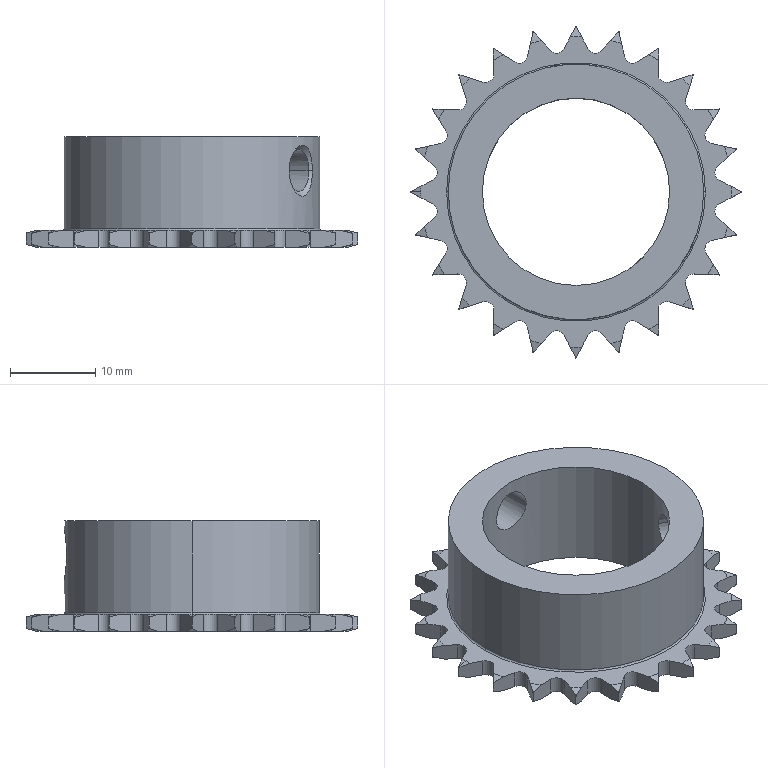Part | SolidWorks | features ICE 3, RevCut 2, Revolution 1 | 1 solid | 197 faces | box 39 x 39 x 13 mm | volume 4619 mm3 | cone 54 | torus 52 | plane 51 | cylinder 40 | commonest cylinder face diameters 2 x32 4.917 x4 22 x2 30 x2